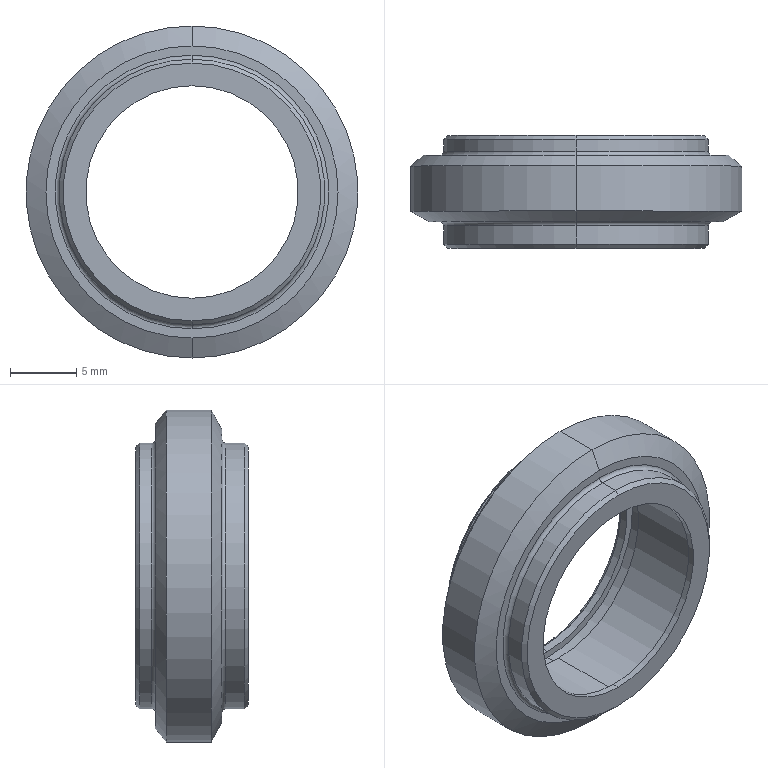Part | STEP file | 1 solid | 35 faces | box 25 x 8.5 x 25 mm | volume 1521 mm3 | cylinder 14 | cone 8 | plane 7 | torus 6 | commonest cylinder face diameters 17 x4 20 x4 16 x2 18.1 x2 25 x2